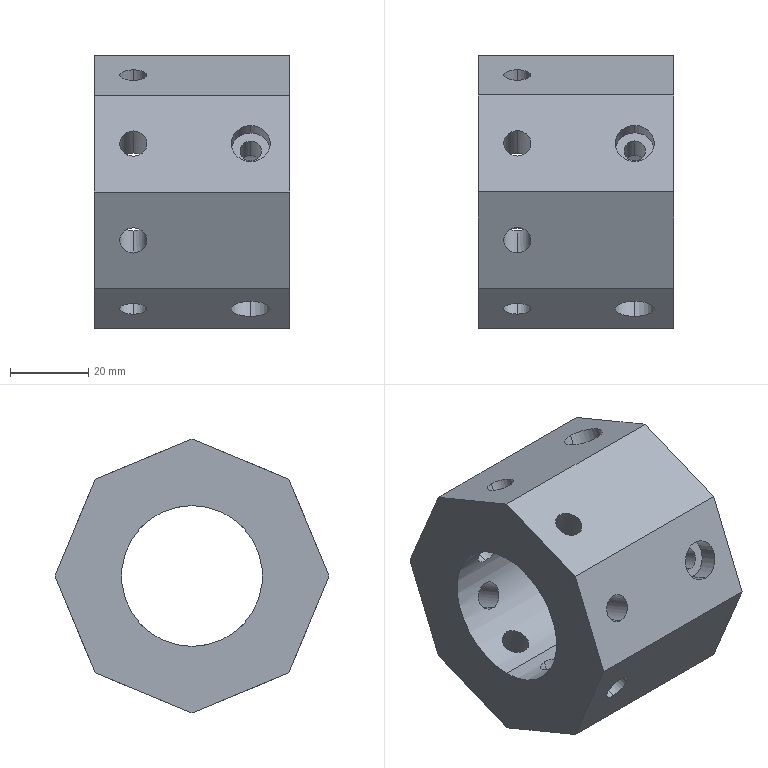Part | SolidWorks | features CirPattern 3, 3DProfileFeature 2, HoleWzd 2, ICE 2, Extrusion 1 | 1 solid | 64 faces | box 50 x 70 x 70 mm | volume 115293 mm3 | cylinder 42 | plane 14 | cone 8 | commonest cylinder face diameters 7 x16 2.5 x8 5.5 x8 10 x8 36 x2